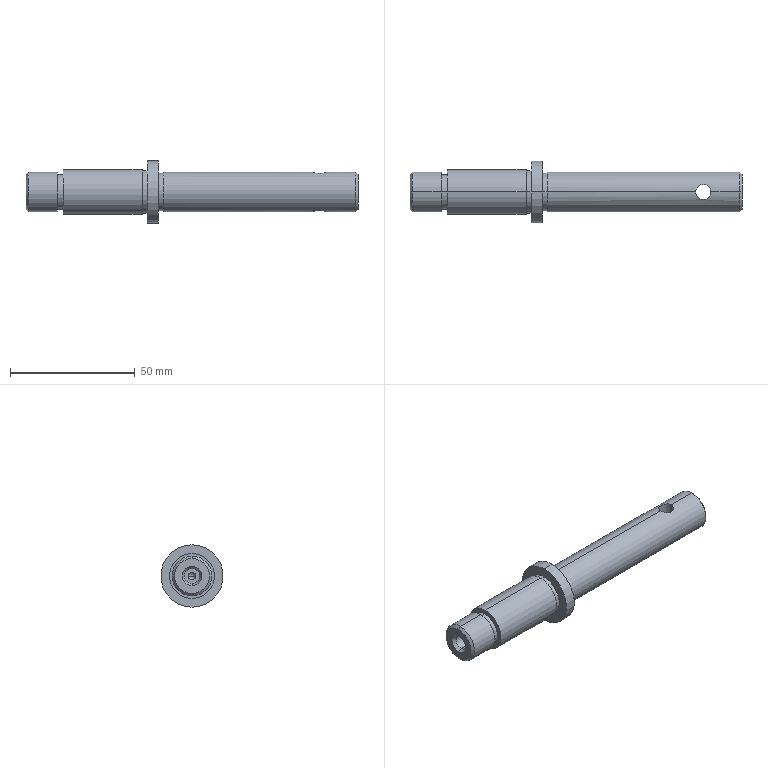Part | SolidWorks | features ICE 3, Chamfer 2, RevCut 1, Revolution 1 | 1 solid | 37 faces | box 133 x 25 x 25 mm | volume 28520 mm3 | cylinder 20 | plane 9 | cone 6 | sphere 2 | commonest cylinder face diameters 6 x4 16 x4 3 x2 14 x2 15 x2 17 x2
STEP:
#1=CARTESIAN_POINT('',(58.,-1.5,0.));
#2=VERTEX_POINT('',#1);
#3=CARTESIAN_POINT('',(58.,0.,-1.5));
#4=VERTEX_POINT('',#3);
#5=CARTESIAN_POINT('',(58.,0.,0.));
#6=DIRECTION('',(1.,0.,0.));
#7=DIRECTION('',(0.,0.,1.));
#8=AXIS2_PLACEMENT_3D('',#5,#6,#7);
#9=CIRCLE('',#8,1.5);
#10=EDGE_CURVE('',#2,#4,#9,.T.);
#11=ORIENTED_EDGE('',*,*,#10,.F.);
#12=CARTESIAN_POINT('',(58.,1.5,0.));
#13=VERTEX_POINT('',#12);
#14=CARTESIAN_POINT('',(58.,0.,0.));
#15=DIRECTION('',(0.,0.,1.));
#16=DIRECTION('',(1.,0.,0.));
#17=AXIS2_PLACEMENT_3D('',#14,#15,#16);
#18=CIRCLE('',#17,1.5);
#19=EDGE_CURVE('',#2,#13,#18,.T.);
#20=ORIENTED_EDGE('',*,*,#19,.T.);
#21=CARTESIAN_POINT('',(58.,0.,0.));
#22=DIRECTION('',(1.,0.,0.));
#23=DIRECTION('',(0.,0.,1.));
#24=AXIS2_PLACEMENT_3D('',#21,#22,#23);
#25=CIRCLE('',#24,1.5);
#26=EDGE_CURVE('',#4,#13,#25,.T.);
#27=ORIENTED_EDGE('',*,*,#26,.F.);
#28=EDGE_LOOP('',(#11,#20,#27));
#29=FACE_OUTER_BOUND('',#28,.T.);
#30=CARTESIAN_POINT('',(58.,0.,0.));
#31=DIRECTION('',(0.,0.,-1.));
#32=DIRECTION('',(1.,0.,0.));
#33=AXIS2_PLACEMENT_3D('',#30,#31,#32);
#34=SPHERICAL_SURFACE('',#33,1.5);
#35=ADVANCED_FACE('',(#29),#34,.F.);
#36=CARTESIAN_POINT('',(0.,0.,7.));
#37=VERTEX_POINT('',#36);
#38=CARTESIAN_POINT('',(0.,0.,-7.));
#39=VERTEX_POINT('',#38);
#40=CARTESIAN_POINT('',(0.,0.,0.));
#41=DIRECTION('',(-1.,0.,0.));
#42=DIRECTION('',(0.,0.,1.));
#43=AXIS2_PLACEMENT_3D('',#40,#41,#42);
#44=CIRCLE('',#43,7.);
#45=EDGE_CURVE('',#37,#39,#44,.T.);
#46=ORIENTED_EDGE('',*,*,#45,.F.);
#47=CARTESIAN_POINT('',(1.,0.,8.));
#48=VERTEX_POINT('',#47);
#49=CARTESIAN_POINT('',(1.,0.,8.));
#50=DIRECTION('',(0.7071,0.,0.7071));
#51=VECTOR('',#50,1000.);
#52=LINE('',#49,#51);
#53=EDGE_CURVE('',#37,#48,#52,.T.);
#54=ORIENTED_EDGE('',*,*,#53,.T.);
#55=CARTESIAN_POINT('',(1.,0.,-8.));
#56=VERTEX_POINT('',#55);
#57=CARTESIAN_POINT('',(1.,0.,0.));
#58=DIRECTION('',(1.,0.,0.));
#59=DIRECTION('',(0.,0.,1.));
#60=AXIS2_PLACEMENT_3D('',#57,#58,#59);
#61=CIRCLE('',#60,8.);
#62=EDGE_CURVE('',#56,#48,#61,.T.);
#63=ORIENTED_EDGE('',*,*,#62,.F.);
#64=CARTESIAN_POINT('',(1.,0.,-8.));
#65=DIRECTION('',(0.7071,0.,-0.7071));
#66=VECTOR('',#65,1000.);
#67=LINE('',#64,#66);
#68=EDGE_CURVE('',#39,#56,#67,.T.);
#69=ORIENTED_EDGE('',*,*,#68,.F.);
#70=EDGE_LOOP('',(#46,#54,#63,#69));
#71=FACE_OUTER_BOUND('',#70,.T.);
#72=CARTESIAN_POINT('',(1.,0.,0.));
#73=DIRECTION('',(1.,0.,0.));
#74=DIRECTION('',(0.,0.,-1.));
#75=AXIS2_PLACEMENT_3D('',#72,#73,#74);
#76=CONICAL_SURFACE('',#75,8.,0.7854);
#77=ADVANCED_FACE('',(#71),#76,.T.);
#78=CARTESIAN_POINT('',(133.,0.,-7.));
#79=VERTEX_POINT('',#78);
#80=CARTESIAN_POINT('',(133.,0.,7.));
#81=VERTEX_POINT('',#80);
#82=CARTESIAN_POINT('',(133.,0.,0.));
#83=DIRECTION('',(1.,0.,0.));
#84=DIRECTION('',(0.,0.,-1.));
#85=AXIS2_PLACEMENT_3D('',#82,#83,#84);
#86=CIRCLE('',#85,7.);
#87=EDGE_CURVE('',#79,#81,#86,.T.);
#88=ORIENTED_EDGE('',*,*,#87,.F.);
#89=CARTESIAN_POINT('',(132.,0.,-8.));
#90=VERTEX_POINT('',#89);
#91=CARTESIAN_POINT('',(133.,0.,-7.));
#92=DIRECTION('',(-0.7071,0.,-0.7071));
#93=VECTOR('',#92,1000.);
#94=LINE('',#91,#93);
#95=EDGE_CURVE('',#79,#90,#94,.T.);
#96=ORIENTED_EDGE('',*,*,#95,.T.);
#97=CARTESIAN_POINT('',(132.,0.,8.));
#98=VERTEX_POINT('',#97);
#99=CARTESIAN_POINT('',(132.,0.,0.));
#100=DIRECTION('',(-1.,0.,0.));
#101=DIRECTION('',(0.,0.,-1.));
#102=AXIS2_PLACEMENT_3D('',#99,#100,#101);
#103=CIRCLE('',#102,8.);
#104=EDGE_CURVE('',#98,#90,#103,.T.);
#105=ORIENTED_EDGE('',*,*,#104,.F.);
#106=CARTESIAN_POINT('',(133.,0.,7.));
#107=DIRECTION('',(-0.7071,0.,0.7071));
#108=VECTOR('',#107,1000.);
#109=LINE('',#106,#108);
#110=EDGE_CURVE('',#81,#98,#109,.T.);
#111=ORIENTED_EDGE('',*,*,#110,.F.);
#112=EDGE_LOOP('',(#88,#96,#105,#111));
#113=FACE_OUTER_BOUND('',#112,.T.);
#114=CARTESIAN_POINT('',(133.,0.,0.));
#115=DIRECTION('',(-1.,0.,0.));
#116=DIRECTION('',(0.,0.,1.));
#117=AXIS2_PLACEMENT_3D('',#114,#115,#116);
#118=CONICAL_SURFACE('',#117,7.,0.7854);
#119=ADVANCED_FACE('',(#113),#118,.T.);
#120=CARTESIAN_POINT('',(1.5,0.,-3.));
#121=VERTEX_POINT('',#120);
#122=CARTESIAN_POINT('',(1.5,0.,3.));
#123=VERTEX_POINT('',#122);
#124=CARTESIAN_POINT('',(1.5,0.,0.));
#125=DIRECTION('',(-1.,0.,0.));
#126=DIRECTION('',(0.,0.,1.));
#127=AXIS2_PLACEMENT_3D('',#124,#125,#126);
#128=CIRCLE('',#127,3.);
#129=EDGE_CURVE('',#121,#123,#128,.T.);
#130=ORIENTED_EDGE('',*,*,#129,.F.);
#131=CARTESIAN_POINT('',(0.,0.,-3.866));
#132=VERTEX_POINT('',#131);
#133=CARTESIAN_POINT('',(0.,0.,-3.866));
#134=DIRECTION('',(-0.866,0.,-0.5));
#135=VECTOR('',#134,1000.);
#136=LINE('',#133,#135);
#137=EDGE_CURVE('',#121,#132,#136,.T.);
#138=ORIENTED_EDGE('',*,*,#137,.T.);
#139=CARTESIAN_POINT('',(0.,0.,3.866));
#140=VERTEX_POINT('',#139);
#141=CARTESIAN_POINT('',(0.,0.,0.));
#142=DIRECTION('',(1.,0.,0.));
#143=DIRECTION('',(0.,0.,1.));
#144=AXIS2_PLACEMENT_3D('',#141,#142,#143);
#145=CIRCLE('',#144,3.866);
#146=EDGE_CURVE('',#140,#132,#145,.T.);
#147=ORIENTED_EDGE('',*,*,#146,.F.);
#148=CARTESIAN_POINT('',(0.,0.,3.866));
#149=DIRECTION('',(-0.866,0.,0.5));
#150=VECTOR('',#149,1000.);
#151=LINE('',#148,#150);
#152=EDGE_CURVE('',#123,#140,#151,.T.);
#153=ORIENTED_EDGE('',*,*,#152,.F.);
#154=EDGE_LOOP('',(#130,#138,#147,#153));
#155=FACE_OUTER_BOUND('',#154,.T.);
#156=CARTESIAN_POINT('',(0.,0.,0.));
#157=DIRECTION('',(-1.,0.,0.));
#158=DIRECTION('',(0.,0.,1.));
#159=AXIS2_PLACEMENT_3D('',#156,#157,#158);
#160=CONICAL_SURFACE('',#159,3.866,0.5236);
#161=ADVANCED_FACE('',(#155),#160,.F.);
#162=CARTESIAN_POINT('',(58.,0.,1.5));
#163=VERTEX_POINT('',#162);
#164=CARTESIAN_POINT('',(58.,0.,0.));
#165=DIRECTION('',(1.,0.,0.));
#166=DIRECTION('',(0.,0.,1.));
#167=AXIS2_PLACEMENT_3D('',#164,#165,#166);
#168=CIRCLE('',#167,1.5);
#169=EDGE_CURVE('',#163,#2,#168,.T.);
#170=ORIENTED_EDGE('',*,*,#169,.T.);
#171=ORIENTED_EDGE('',*,*,#10,.T.);
#172=CARTESIAN_POINT('',(8.,0.,-1.5));
#173=VERTEX_POINT('',#172);
#174=CARTESIAN_POINT('',(58.,0.,-1.5));
#175=DIRECTION('',(-1.,0.,0.));
#176=VECTOR('',#175,1000.);
#177=LINE('',#174,#176);
#178=EDGE_CURVE('',#4,#173,#177,.T.);
#179=ORIENTED_EDGE('',*,*,#178,.T.);
#180=CARTESIAN_POINT('',(8.,0.,1.5));
#181=VERTEX_POINT('',#180);
#182=CARTESIAN_POINT('',(8.,0.,0.));
#183=DIRECTION('',(-1.,0.,0.));
#184=DIRECTION('',(0.,0.,1.));
#185=AXIS2_PLACEMENT_3D('',#182,#183,#184);
#186=CIRCLE('',#185,1.5);
#187=EDGE_CURVE('',#173,#181,#186,.T.);
#188=ORIENTED_EDGE('',*,*,#187,.T.);
#189=CARTESIAN_POINT('',(58.,0.,1.5));
#190=DIRECTION('',(-1.,0.,0.));
#191=VECTOR('',#190,1000.);
#192=LINE('',#189,#191);
#193=EDGE_CURVE('',#163,#181,#192,.T.);
#194=ORIENTED_EDGE('',*,*,#193,.F.);
#195=EDGE_LOOP('',(#170,#171,#179,#188,#194));
#196=FACE_OUTER_BOUND('',#195,.T.);
#197=CARTESIAN_POINT('',(58.,0.,0.));
#198=DIRECTION('',(-1.,0.,0.));
#199=DIRECTION('',(0.,0.,1.));
#200=AXIS2_PLACEMENT_3D('',#197,#198,#199);
#201=CYLINDRICAL_SURFACE('',#200,1.5);
#202=ADVANCED_FACE('',(#196),#201,.F.);
#203=ORIENTED_EDGE('',*,*,#129,.T.);
#204=CARTESIAN_POINT('',(8.,0.,3.));
#205=VERTEX_POINT('',#204);
#206=CARTESIAN_POINT('',(-0.000012,0.,3.));
#207=DIRECTION('',(1.,0.,0.));
#208=VECTOR('',#207,1000.);
#209=LINE('',#206,#208);
#210=EDGE_CURVE('',#123,#205,#209,.T.);
#211=ORIENTED_EDGE('',*,*,#210,.T.);
#212=CARTESIAN_POINT('',(8.,0.,-3.));
#213=VERTEX_POINT('',#212);
#214=CARTESIAN_POINT('',(8.,0.,0.));
#215=DIRECTION('',(-1.,0.,0.));
#216=DIRECTION('',(0.,0.,1.));
#217=AXIS2_PLACEMENT_3D('',#214,#215,#216);
#218=CIRCLE('',#217,3.);
#219=EDGE_CURVE('',#213,#205,#218,.T.);
#220=ORIENTED_EDGE('',*,*,#219,.F.);
#221=CARTESIAN_POINT('',(-0.000012,0.,-3.));
#222=DIRECTION('',(1.,0.,0.));
#223=VECTOR('',#222,1000.);
#224=LINE('',#221,#223);
#225=EDGE_CURVE('',#121,#213,#224,.T.);
#226=ORIENTED_EDGE('',*,*,#225,.F.);
#227=EDGE_LOOP('',(#203,#211,#220,#226));
#228=FACE_OUTER_BOUND('',#227,.T.);
#229=CARTESIAN_POINT('',(-0.000012,0.,0.));
#230=DIRECTION('',(1.,0.,0.));
#231=DIRECTION('',(0.,0.,-1.));
#232=AXIS2_PLACEMENT_3D('',#229,#230,#231);
#233=CYLINDRICAL_SURFACE('',#232,3.);
#234=ADVANCED_FACE('',(#228),#233,.F.);
#235=CARTESIAN_POINT('',(120.5,0.,-8.));
#236=VERTEX_POINT('',#235);
#237=CARTESIAN_POINT('',(114.5,0.,-8.));
#238=VERTEX_POINT('',#237);
#239=CARTESIAN_POINT('',(120.5,0.,-8.));
#240=CARTESIAN_POINT('',(120.5,-0.1971,-8.));
#241=CARTESIAN_POINT('',(120.48,-0.3965,-7.993));
#242=CARTESIAN_POINT('',(120.402,-0.7855,-7.964));
#243=CARTESIAN_POINT('',(120.345,-0.9732,-7.943));
#244=CARTESIAN_POINT('',(120.193,-1.336,-7.89));
#245=CARTESIAN_POINT('',(120.099,-1.511,-7.858));
#246=CARTESIAN_POINT('',(119.882,-1.834,-7.789));
#247=CARTESIAN_POINT('',(119.759,-1.984,-7.751));
#248=CARTESIAN_POINT('',(119.481,-2.261,-7.675));
#249=CARTESIAN_POINT('',(119.331,-2.385,-7.637));
#250=CARTESIAN_POINT('',(119.008,-2.601,-7.566));
#251=CARTESIAN_POINT('',(118.834,-2.694,-7.533));
#252=CARTESIAN_POINT('',(118.471,-2.845,-7.477));
#253=CARTESIAN_POINT('',(118.283,-2.903,-7.455));
#254=CARTESIAN_POINT('',(117.897,-2.98,-7.424));
#255=CARTESIAN_POINT('',(117.696,-3.,-7.416));
#256=CARTESIAN_POINT('',(117.301,-3.,-7.416));
#257=CARTESIAN_POINT('',(117.105,-2.98,-7.424));
#258=CARTESIAN_POINT('',(116.715,-2.902,-7.455));
#259=CARTESIAN_POINT('',(116.525,-2.844,-7.478));
#260=CARTESIAN_POINT('',(116.164,-2.693,-7.533));
#261=CARTESIAN_POINT('',(115.99,-2.6,-7.567));
#262=CARTESIAN_POINT('',(115.665,-2.382,-7.638));
#263=CARTESIAN_POINT('',(115.516,-2.258,-7.676));
#264=CARTESIAN_POINT('',(115.241,-1.983,-7.752));
#265=CARTESIAN_POINT('',(115.115,-1.83,-7.79));
#266=CARTESIAN_POINT('',(114.899,-1.507,-7.859));
#267=CARTESIAN_POINT('',(114.806,-1.336,-7.89));
#268=CARTESIAN_POINT('',(114.655,-0.9711,-7.943));
#269=CARTESIAN_POINT('',(114.597,-0.781,-7.964));
#270=CARTESIAN_POINT('',(114.52,-0.3964,-7.992));
#271=CARTESIAN_POINT('',(114.5,-0.2002,-8.));
#272=CARTESIAN_POINT('',(114.5,0.,-8.));
#273=B_SPLINE_CURVE_WITH_KNOTS('',3,(#239,#240,#241,#242,#243,#244,#245,#246,#247,#248,#249,#250,#251,#252,#253,#254,#255,#256,#257,#258,#259,#260,#261,#262,#263,#264,#265,#266,#267,#268,#269,#270,#271,#272),.UNSPECIFIED.,.F.,.F.,(4,2,2,2,2,2,2,2,2,2,2,2,2,2,2,2,4),(0.009467,0.01006,0.01065,0.01124,0.01183,0.01242,0.01302,0.01361,0.0142,0.01479,0.01538,0.01597,0.01657,0.01716,0.01775,0.01834,0.01893),.UNSPECIFIED.);
#274=EDGE_CURVE('',#236,#238,#273,.T.);
#275=ORIENTED_EDGE('',*,*,#274,.T.);
#276=CARTESIAN_POINT('',(114.5,0.,8.));
#277=VERTEX_POINT('',#276);
#278=CARTESIAN_POINT('',(114.5,0.,-12.5));
#279=DIRECTION('',(0.,0.,1.));
#280=VECTOR('',#279,1000.);
#281=LINE('',#278,#280);
#282=EDGE_CURVE('',#238,#277,#281,.T.);
#283=ORIENTED_EDGE('',*,*,#282,.T.);
#284=CARTESIAN_POINT('',(120.5,0.,8.));
#285=VERTEX_POINT('',#284);
#286=CARTESIAN_POINT('',(114.5,0.,8.));
#287=CARTESIAN_POINT('',(114.5,-0.1971,8.));
#288=CARTESIAN_POINT('',(114.52,-0.3965,7.993));
#289=CARTESIAN_POINT('',(114.598,-0.7855,7.964));
#290=CARTESIAN_POINT('',(114.655,-0.9732,7.943));
#291=CARTESIAN_POINT('',(114.807,-1.336,7.89));
#292=CARTESIAN_POINT('',(114.901,-1.511,7.858));
#293=CARTESIAN_POINT('',(115.118,-1.834,7.789));
#294=CARTESIAN_POINT('',(115.241,-1.984,7.751));
#295=CARTESIAN_POINT('',(115.519,-2.261,7.675));
#296=CARTESIAN_POINT('',(115.669,-2.385,7.637));
#297=CARTESIAN_POINT('',(115.992,-2.601,7.566));
#298=CARTESIAN_POINT('',(116.166,-2.694,7.533));
#299=CARTESIAN_POINT('',(116.529,-2.845,7.477));
#300=CARTESIAN_POINT('',(116.717,-2.903,7.455));
#301=CARTESIAN_POINT('',(117.103,-2.98,7.424));
#302=CARTESIAN_POINT('',(117.304,-3.,7.416));
#303=CARTESIAN_POINT('',(117.699,-3.,7.416));
#304=CARTESIAN_POINT('',(117.895,-2.98,7.424));
#305=CARTESIAN_POINT('',(118.285,-2.902,7.455));
#306=CARTESIAN_POINT('',(118.475,-2.844,7.478));
#307=CARTESIAN_POINT('',(118.836,-2.693,7.533));
#308=CARTESIAN_POINT('',(119.01,-2.6,7.567));
#309=CARTESIAN_POINT('',(119.335,-2.382,7.638));
#310=CARTESIAN_POINT('',(119.484,-2.258,7.676));
#311=CARTESIAN_POINT('',(119.759,-1.983,7.752));
#312=CARTESIAN_POINT('',(119.885,-1.83,7.79));
#313=CARTESIAN_POINT('',(120.101,-1.507,7.859));
#314=CARTESIAN_POINT('',(120.194,-1.336,7.89));
#315=CARTESIAN_POINT('',(120.345,-0.9711,7.943));
#316=CARTESIAN_POINT('',(120.403,-0.781,7.964));
#317=CARTESIAN_POINT('',(120.48,-0.3964,7.992));
#318=CARTESIAN_POINT('',(120.5,-0.2002,8.));
#319=CARTESIAN_POINT('',(120.5,0.,8.));
#320=B_SPLINE_CURVE_WITH_KNOTS('',3,(#286,#287,#288,#289,#290,#291,#292,#293,#294,#295,#296,#297,#298,#299,#300,#301,#302,#303,#304,#305,#306,#307,#308,#309,#310,#311,#312,#313,#314,#315,#316,#317,#318,#319),.UNSPECIFIED.,.F.,.F.,(4,2,2,2,2,2,2,2,2,2,2,2,2,2,2,2,4),(0.009467,0.01006,0.01065,0.01124,0.01183,0.01242,0.01302,0.01361,0.0142,0.01479,0.01538,0.01597,0.01657,0.01716,0.01775,0.01834,0.01893),.UNSPECIFIED.);
#321=EDGE_CURVE('',#277,#285,#320,.T.);
#322=ORIENTED_EDGE('',*,*,#321,.T.);
#323=CARTESIAN_POINT('',(120.5,0.,-12.5));
#324=DIRECTION('',(0.,0.,1.));
#325=VECTOR('',#324,1000.);
#326=LINE('',#323,#325);
#327=EDGE_CURVE('',#236,#285,#326,.T.);
#328=ORIENTED_EDGE('',*,*,#327,.F.);
#329=EDGE_LOOP('',(#275,#283,#322,#328));
#330=FACE_OUTER_BOUND('',#329,.T.);
#331=CARTESIAN_POINT('',(117.5,0.,-12.5));
#332=DIRECTION('',(0.,0.,1.));
#333=DIRECTION('',(1.,0.,0.));
#334=AXIS2_PLACEMENT_3D('',#331,#332,#333);
#335=CYLINDRICAL_SURFACE('',#334,3.);
#336=ADVANCED_FACE('',(#330),#335,.F.);
#337=CARTESIAN_POINT('',(55.,0.,-8.));
#338=VERTEX_POINT('',#337);
#339=CARTESIAN_POINT('',(55.,0.,8.));
#340=VERTEX_POINT('',#339);
#341=CARTESIAN_POINT('',(55.,0.,0.));
#342=DIRECTION('',(1.,0.,0.));
#343=DIRECTION('',(0.,0.,-1.));
#344=AXIS2_PLACEMENT_3D('',#341,#342,#343);
#345=CIRCLE('',#344,8.);
#346=EDGE_CURVE('',#338,#340,#345,.T.);
#347=ORIENTED_EDGE('',*,*,#346,.T.);
#348=CARTESIAN_POINT('',(133.,0.,8.));
#349=DIRECTION('',(1.,0.,0.));
#350=VECTOR('',#349,1000.);
#351=LINE('',#348,#350);
#352=EDGE_CURVE('',#340,#277,#351,.T.);
#353=ORIENTED_EDGE('',*,*,#352,.T.);
#354=CARTESIAN_POINT('',(120.5,0.,8.));
#355=CARTESIAN_POINT('',(120.5,0.2002,8.));
#356=CARTESIAN_POINT('',(120.48,0.3967,7.993));
#357=CARTESIAN_POINT('',(120.403,0.7827,7.964));
#358=CARTESIAN_POINT('',(120.344,0.9743,7.943));
#359=CARTESIAN_POINT('',(120.193,1.337,7.89));
#360=CARTESIAN_POINT('',(120.1,1.509,7.858));
#361=CARTESIAN_POINT('',(119.883,1.833,7.789));
#362=CARTESIAN_POINT('',(119.757,1.986,7.751));
#363=CARTESIAN_POINT('',(119.346,2.396,7.638));
#364=CARTESIAN_POINT('',(119.015,2.619,7.561));
#365=CARTESIAN_POINT('',(118.474,2.844,7.478));
#366=CARTESIAN_POINT('',(118.283,2.903,7.455));
#367=CARTESIAN_POINT('',(117.895,2.98,7.424));
#368=CARTESIAN_POINT('',(117.699,3.,7.416));
#369=CARTESIAN_POINT('',(117.304,3.,7.416));
#370=CARTESIAN_POINT('',(117.103,2.98,7.424));
#371=CARTESIAN_POINT('',(116.717,2.903,7.455));
#372=CARTESIAN_POINT('',(116.529,2.845,7.477));
#373=CARTESIAN_POINT('',(116.163,2.693,7.534));
#374=CARTESIAN_POINT('',(115.991,2.6,7.566));
#375=CARTESIAN_POINT('',(115.668,2.384,7.637));
#376=CARTESIAN_POINT('',(115.515,2.258,7.676));
#377=CARTESIAN_POINT('',(115.24,1.983,7.752));
#378=CARTESIAN_POINT('',(115.117,1.833,7.789));
#379=CARTESIAN_POINT('',(114.9,1.509,7.858));
#380=CARTESIAN_POINT('',(114.806,1.334,7.89));
#381=CARTESIAN_POINT('',(114.655,0.973,7.943));
#382=CARTESIAN_POINT('',(114.598,0.7855,7.964));
#383=CARTESIAN_POINT('',(114.52,0.3956,7.993));
#384=CARTESIAN_POINT('',(114.5,0.1972,8.));
#385=CARTESIAN_POINT('',(114.5,0.,8.));
#386=B_SPLINE_CURVE_WITH_KNOTS('',3,(#354,#355,#356,#357,#358,#359,#360,#361,#362,#363,#364,#365,#366,#367,#368,#369,#370,#371,#372,#373,#374,#375,#376,#377,#378,#379,#380,#381,#382,#383,#384,#385),.UNSPECIFIED.,.F.,.F.,(4,2,2,2,2,2,2,2,2,2,2,2,2,2,2,4),(0.,0.0005917,0.001183,0.001775,0.002367,0.00355,0.004142,0.004733,0.005325,0.005917,0.006508,0.0071,0.007692,0.008283,0.008875,0.009467),.UNSPECIFIED.);
#387=EDGE_CURVE('',#285,#277,#386,.T.);
#388=ORIENTED_EDGE('',*,*,#387,.F.);
#389=CARTESIAN_POINT('',(133.,0.,8.));
#390=DIRECTION('',(1.,0.,0.));
#391=VECTOR('',#390,1000.);
#392=LINE('',#389,#391);
#393=EDGE_CURVE('',#285,#98,#392,.T.);
#394=ORIENTED_EDGE('',*,*,#393,.T.);
#395=ORIENTED_EDGE('',*,*,#104,.T.);
#396=CARTESIAN_POINT('',(133.,0.,-8.));
#397=DIRECTION('',(1.,0.,0.));
#398=VECTOR('',#397,1000.);
#399=LINE('',#396,#398);
#400=EDGE_CURVE('',#236,#90,#399,.T.);
#401=ORIENTED_EDGE('',*,*,#400,.F.);
#402=CARTESIAN_POINT('',(114.5,0.,-8.));
#403=CARTESIAN_POINT('',(114.5,0.2002,-8.));
#404=CARTESIAN_POINT('',(114.52,0.3967,-7.993));
#405=CARTESIAN_POINT('',(114.597,0.7827,-7.964));
#406=CARTESIAN_POINT('',(114.656,0.9743,-7.943));
#407=CARTESIAN_POINT('',(114.807,1.337,-7.89));
#408=CARTESIAN_POINT('',(114.9,1.509,-7.858));
#409=CARTESIAN_POINT('',(115.117,1.833,-7.789));
#410=CARTESIAN_POINT('',(115.243,1.986,-7.751));
#411=CARTESIAN_POINT('',(115.654,2.396,-7.638));
#412=CARTESIAN_POINT('',(115.985,2.619,-7.561));
#413=CARTESIAN_POINT('',(116.526,2.844,-7.478));
#414=CARTESIAN_POINT('',(116.717,2.903,-7.455));
#415=CARTESIAN_POINT('',(117.105,2.98,-7.424));
#416=CARTESIAN_POINT('',(117.301,3.,-7.416));
#417=CARTESIAN_POINT('',(117.696,3.,-7.416));
#418=CARTESIAN_POINT('',(117.897,2.98,-7.424));
#419=CARTESIAN_POINT('',(118.283,2.903,-7.455));
#420=CARTESIAN_POINT('',(118.471,2.845,-7.477));
#421=CARTESIAN_POINT('',(118.837,2.693,-7.534));
#422=CARTESIAN_POINT('',(119.009,2.6,-7.566));
#423=CARTESIAN_POINT('',(119.332,2.384,-7.637));
#424=CARTESIAN_POINT('',(119.485,2.258,-7.676));
#425=CARTESIAN_POINT('',(119.76,1.983,-7.752));
#426=CARTESIAN_POINT('',(119.883,1.833,-7.789));
#427=CARTESIAN_POINT('',(120.1,1.509,-7.858));
#428=CARTESIAN_POINT('',(120.194,1.334,-7.89));
#429=CARTESIAN_POINT('',(120.345,0.973,-7.943));
#430=CARTESIAN_POINT('',(120.402,0.7855,-7.964));
#431=CARTESIAN_POINT('',(120.48,0.3956,-7.993));
#432=CARTESIAN_POINT('',(120.5,0.1972,-8.));
#433=CARTESIAN_POINT('',(120.5,0.,-8.));
#434=B_SPLINE_CURVE_WITH_KNOTS('',3,(#402,#403,#404,#405,#406,#407,#408,#409,#410,#411,#412,#413,#414,#415,#416,#417,#418,#419,#420,#421,#422,#423,#424,#425,#426,#427,#428,#429,#430,#431,#432,#433),.UNSPECIFIED.,.F.,.F.,(4,2,2,2,2,2,2,2,2,2,2,2,2,2,2,4),(0.,0.0005917,0.001183,0.001775,0.002367,0.00355,0.004142,0.004733,0.005325,0.005917,0.006508,0.0071,0.007692,0.008283,0.008875,0.009467),.UNSPECIFIED.);
#435=EDGE_CURVE('',#238,#236,#434,.T.);
#436=ORIENTED_EDGE('',*,*,#435,.F.);
#437=CARTESIAN_POINT('',(133.,0.,-8.));
#438=DIRECTION('',(1.,0.,0.));
#439=VECTOR('',#438,1000.);
#440=LINE('',#437,#439);
#441=EDGE_CURVE('',#338,#238,#440,.T.);
#442=ORIENTED_EDGE('',*,*,#441,.F.);
#443=EDGE_LOOP('',(#347,#353,#388,#394,#395,#401,#436,#442));
#444=FACE_OUTER_BOUND('',#443,.T.);
#445=CARTESIAN_POINT('',(133.,0.,0.));
#446=DIRECTION('',(1.,0.,0.));
#447=DIRECTION('',(0.,0.,-1.));
#448=AXIS2_PLACEMENT_3D('',#445,#446,#447);
#449=CYLINDRICAL_SURFACE('',#448,8.);
#450=ADVANCED_FACE('',(#444),#449,.T.);
#451=CARTESIAN_POINT('',(53.,0.,-7.5));
#452=VERTEX_POINT('',#451);
#453=CARTESIAN_POINT('',(53.,0.,7.5));
#454=VERTEX_POINT('',#453);
#455=CARTESIAN_POINT('',(53.,0.,0.));
#456=DIRECTION('',(1.,0.,0.));
#457=DIRECTION('',(0.,0.,-1.));
#458=AXIS2_PLACEMENT_3D('',#455,#456,#457);
#459=CIRCLE('',#458,7.5);
#460=EDGE_CURVE('',#452,#454,#459,.T.);
#461=ORIENTED_EDGE('',*,*,#460,.T.);
#462=CARTESIAN_POINT('',(55.,0.,7.5));
#463=VERTEX_POINT('',#462);
#464=CARTESIAN_POINT('',(133.,0.,7.5));
#465=DIRECTION('',(1.,0.,0.));
#466=VECTOR('',#465,1000.);
#467=LINE('',#464,#466);
#468=EDGE_CURVE('',#454,#463,#467,.T.);
#469=ORIENTED_EDGE('',*,*,#468,.T.);
#470=CARTESIAN_POINT('',(55.,0.,-7.5));
#471=VERTEX_POINT('',#470);
#472=CARTESIAN_POINT('',(55.,0.,0.));
#473=DIRECTION('',(1.,0.,0.));
#474=DIRECTION('',(0.,0.,-1.));
#475=AXIS2_PLACEMENT_3D('',#472,#473,#474);
#476=CIRCLE('',#475,7.5);
#477=EDGE_CURVE('',#471,#463,#476,.T.);
#478=ORIENTED_EDGE('',*,*,#477,.F.);
#479=CARTESIAN_POINT('',(133.,0.,-7.5));
#480=DIRECTION('',(1.,0.,0.));
#481=VECTOR('',#480,1000.);
#482=LINE('',#479,#481);
#483=EDGE_CURVE('',#452,#471,#482,.T.);
#484=ORIENTED_EDGE('',*,*,#483,.F.);
#485=EDGE_LOOP('',(#461,#469,#478,#484));
#486=FACE_OUTER_BOUND('',#485,.T.);
#487=CARTESIAN_POINT('',(133.,0.,0.));
#488=DIRECTION('',(1.,0.,0.));
#489=DIRECTION('',(0.,0.,-1.));
#490=AXIS2_PLACEMENT_3D('',#487,#488,#489);
#491=CYLINDRICAL_SURFACE('',#490,7.5);
#492=ADVANCED_FACE('',(#486),#491,.T.);
#493=CARTESIAN_POINT('',(48.5,0.,-12.5));
#494=VERTEX_POINT('',#493);
#495=CARTESIAN_POINT('',(48.5,0.,12.5));
#496=VERTEX_POINT('',#495);
#497=CARTESIAN_POINT('',(48.5,0.,0.));
#498=DIRECTION('',(1.,0.,0.));
#499=DIRECTION('',(0.,0.,-1.));
#500=AXIS2_PLACEMENT_3D('',#497,#498,#499);
#501=CIRCLE('',#500,12.5);
#502=EDGE_CURVE('',#494,#496,#501,.T.);
#503=ORIENTED_EDGE('',*,*,#502,.T.);
#504=CARTESIAN_POINT('',(53.,0.,12.5));
#505=VERTEX_POINT('',#504);
#506=CARTESIAN_POINT('',(133.,0.,12.5));
#507=DIRECTION('',(1.,0.,0.));
#508=VECTOR('',#507,1000.);
#509=LINE('',#506,#508);
#510=EDGE_CURVE('',#496,#505,#509,.T.);
#511=ORIENTED_EDGE('',*,*,#510,.T.);
#512=CARTESIAN_POINT('',(53.,0.,-12.5));
#513=VERTEX_POINT('',#512);
#514=CARTESIAN_POINT('',(53.,0.,0.));
#515=DIRECTION('',(1.,0.,0.));
#516=DIRECTION('',(0.,0.,-1.));
#517=AXIS2_PLACEMENT_3D('',#514,#515,#516);
#518=CIRCLE('',#517,12.5);
#519=EDGE_CURVE('',#513,#505,#518,.T.);
#520=ORIENTED_EDGE('',*,*,#519,.F.);
#521=CARTESIAN_POINT('',(133.,0.,-12.5));
#522=DIRECTION('',(1.,0.,0.));
#523=VECTOR('',#522,1000.);
#524=LINE('',#521,#523);
#525=EDGE_CURVE('',#494,#513,#524,.T.);
#526=ORIENTED_EDGE('',*,*,#525,.F.);
#527=EDGE_LOOP('',(#503,#511,#520,#526));
#528=FACE_OUTER_BOUND('',#527,.T.);
#529=CARTESIAN_POINT('',(133.,0.,0.));
#530=DIRECTION('',(1.,0.,0.));
#531=DIRECTION('',(0.,0.,-1.));
#532=AXIS2_PLACEMENT_3D('',#529,#530,#531);
#533=CYLINDRICAL_SURFACE('',#532,12.5);
#534=ADVANCED_FACE('',(#528),#533,.T.);
#535=CARTESIAN_POINT('',(46.5,0.,-8.5));
#536=VERTEX_POINT('',#535);
#537=CARTESIAN_POINT('',(46.5,0.,8.5));
#538=VERTEX_POINT('',#537);
#539=CARTESIAN_POINT('',(46.5,0.,0.));
#540=DIRECTION('',(1.,0.,0.));
#541=DIRECTION('',(0.,0.,-1.));
#542=AXIS2_PLACEMENT_3D('',#539,#540,#541);
#543=CIRCLE('',#542,8.5);
#544=EDGE_CURVE('',#536,#538,#543,.T.);
#545=ORIENTED_EDGE('',*,*,#544,.T.);
#546=CARTESIAN_POINT('',(48.5,0.,8.5));
#547=VERTEX_POINT('',#546);
#548=CARTESIAN_POINT('',(133.,0.,8.5));
#549=DIRECTION('',(1.,0.,0.));
#550=VECTOR('',#549,1000.);
#551=LINE('',#548,#550);
#552=EDGE_CURVE('',#538,#547,#551,.T.);
#553=ORIENTED_EDGE('',*,*,#552,.T.);
#554=CARTESIAN_POINT('',(48.5,0.,-8.5));
#555=VERTEX_POINT('',#554);
#556=CARTESIAN_POINT('',(48.5,0.,0.));
#557=DIRECTION('',(1.,0.,0.));
#558=DIRECTION('',(0.,0.,-1.));
#559=AXIS2_PLACEMENT_3D('',#556,#557,#558);
#560=CIRCLE('',#559,8.5);
#561=EDGE_CURVE('',#555,#547,#560,.T.);
#562=ORIENTED_EDGE('',*,*,#561,.F.);
#563=CARTESIAN_POINT('',(133.,0.,-8.5));
#564=DIRECTION('',(1.,0.,0.));
#565=VECTOR('',#564,1000.);
#566=LINE('',#563,#565);
#567=EDGE_CURVE('',#536,#555,#566,.T.);
#568=ORIENTED_EDGE('',*,*,#567,.F.);
#569=EDGE_LOOP('',(#545,#553,#562,#568));
#570=FACE_OUTER_BOUND('',#569,.T.);
#571=CARTESIAN_POINT('',(133.,0.,0.));
#572=DIRECTION('',(1.,0.,0.));
#573=DIRECTION('',(0.,0.,-1.));
#574=AXIS2_PLACEMENT_3D('',#571,#572,#573);
#575=CYLINDRICAL_SURFACE('',#574,8.5);
#576=ADVANCED_FACE('',(#570),#575,.T.);
#577=CARTESIAN_POINT('',(15.,0.,-9.));
#578=VERTEX_POINT('',#577);
#579=CARTESIAN_POINT('',(15.,0.,9.));
#580=VERTEX_POINT('',#579);
#581=CARTESIAN_POINT('',(15.,0.,0.));
#582=DIRECTION('',(1.,0.,0.));
#583=DIRECTION('',(0.,0.,-1.));
#584=AXIS2_PLACEMENT_3D('',#581,#582,#583);
#585=CIRCLE('',#584,9.);
#586=EDGE_CURVE('',#578,#580,#585,.T.);
#587=ORIENTED_EDGE('',*,*,#586,.T.);
#588=CARTESIAN_POINT('',(46.5,0.,9.));
#589=VERTEX_POINT('',#588);
#590=CARTESIAN_POINT('',(133.,0.,9.));
#591=DIRECTION('',(1.,0.,0.));
#592=VECTOR('',#591,1000.);
#593=LINE('',#590,#592);
#594=EDGE_CURVE('',#580,#589,#593,.T.);
#595=ORIENTED_EDGE('',*,*,#594,.T.);
#596=CARTESIAN_POINT('',(46.5,0.,-9.));
#597=VERTEX_POINT('',#596);
#598=CARTESIAN_POINT('',(46.5,0.,0.));
#599=DIRECTION('',(1.,0.,0.));
#600=DIRECTION('',(0.,0.,-1.));
#601=AXIS2_PLACEMENT_3D('',#598,#599,#600);
#602=CIRCLE('',#601,9.);
#603=EDGE_CURVE('',#597,#589,#602,.T.);
#604=ORIENTED_EDGE('',*,*,#603,.F.);
#605=CARTESIAN_POINT('',(133.,0.,-9.));
#606=DIRECTION('',(1.,0.,0.));
#607=VECTOR('',#606,1000.);
#608=LINE('',#605,#607);
#609=EDGE_CURVE('',#578,#597,#608,.T.);
#610=ORIENTED_EDGE('',*,*,#609,.F.);
#611=EDGE_LOOP('',(#587,#595,#604,#610));
#612=FACE_OUTER_BOUND('',#611,.T.);
#613=CARTESIAN_POINT('',(133.,0.,0.));
#614=DIRECTION('',(1.,0.,0.));
#615=DIRECTION('',(0.,0.,-1.));
#616=AXIS2_PLACEMENT_3D('',#613,#614,#615);
#617=CYLINDRICAL_SURFACE('',#616,9.);
#618=ADVANCED_FACE('',(#612),#617,.T.);
#619=CARTESIAN_POINT('',(12.5,0.,-7.));
#620=VERTEX_POINT('',#619);
#621=CARTESIAN_POINT('',(12.5,0.,7.));
#622=VERTEX_POINT('',#621);
#623=CARTESIAN_POINT('',(12.5,0.,0.));
#624=DIRECTION('',(1.,0.,0.));
#625=DIRECTION('',(0.,0.,-1.));
#626=AXIS2_PLACEMENT_3D('',#623,#624,#625);
#627=CIRCLE('',#626,7.);
#628=EDGE_CURVE('',#620,#622,#627,.T.);
#629=ORIENTED_EDGE('',*,*,#628,.T.);
#630=CARTESIAN_POINT('',(15.,0.,7.));
#631=VERTEX_POINT('',#630);
#632=CARTESIAN_POINT('',(133.,0.,7.));
#633=DIRECTION('',(1.,0.,0.));
#634=VECTOR('',#633,1000.);
#635=LINE('',#632,#634);
#636=EDGE_CURVE('',#622,#631,#635,.T.);
#637=ORIENTED_EDGE('',*,*,#636,.T.);
#638=CARTESIAN_POINT('',(15.,0.,-7.));
#639=VERTEX_POINT('',#638);
#640=CARTESIAN_POINT('',(15.,0.,0.));
#641=DIRECTION('',(1.,0.,0.));
#642=DIRECTION('',(0.,0.,-1.));
#643=AXIS2_PLACEMENT_3D('',#640,#641,#642);
#644=CIRCLE('',#643,7.);
#645=EDGE_CURVE('',#639,#631,#644,.T.);
#646=ORIENTED_EDGE('',*,*,#645,.F.);
#647=CARTESIAN_POINT('',(133.,0.,-7.));
#648=DIRECTION('',(1.,0.,0.));
#649=VECTOR('',#648,1000.);
#650=LINE('',#647,#649);
#651=EDGE_CURVE('',#620,#639,#650,.T.);
#652=ORIENTED_EDGE('',*,*,#651,.F.);
#653=EDGE_LOOP('',(#629,#637,#646,#652));
#654=FACE_OUTER_BOUND('',#653,.T.);
#655=CARTESIAN_POINT('',(133.,0.,0.));
#656=DIRECTION('',(1.,0.,0.));
#657=DIRECTION('',(0.,0.,-1.));
#658=AXIS2_PLACEMENT_3D('',#655,#656,#657);
#659=CYLINDRICAL_SURFACE('',#658,7.);
#660=ADVANCED_FACE('',(#654),#659,.T.);
#661=ORIENTED_EDGE('',*,*,#62,.T.);
#662=CARTESIAN_POINT('',(12.5,0.,8.));
#663=VERTEX_POINT('',#662);
#664=CARTESIAN_POINT('',(133.,0.,8.));
#665=DIRECTION('',(1.,0.,0.));
#666=VECTOR('',#665,1000.);
#667=LINE('',#664,#666);
#668=EDGE_CURVE('',#48,#663,#667,.T.);
#669=ORIENTED_EDGE('',*,*,#668,.T.);
#670=CARTESIAN_POINT('',(12.5,0.,-8.));
#671=VERTEX_POINT('',#670);
#672=CARTESIAN_POINT('',(12.5,0.,0.));
#673=DIRECTION('',(1.,0.,0.));
#674=DIRECTION('',(0.,0.,-1.));
#675=AXIS2_PLACEMENT_3D('',#672,#673,#674);
#676=CIRCLE('',#675,8.);
#677=EDGE_CURVE('',#671,#663,#676,.T.);
#678=ORIENTED_EDGE('',*,*,#677,.F.);
#679=CARTESIAN_POINT('',(133.,0.,-8.));
#680=DIRECTION('',(1.,0.,0.));
#681=VECTOR('',#680,1000.);
#682=LINE('',#679,#681);
#683=EDGE_CURVE('',#56,#671,#682,.T.);
#684=ORIENTED_EDGE('',*,*,#683,.F.);
#685=EDGE_LOOP('',(#661,#669,#678,#684));
#686=FACE_OUTER_BOUND('',#685,.T.);
#687=CARTESIAN_POINT('',(133.,0.,0.));
#688=DIRECTION('',(1.,0.,0.));
#689=DIRECTION('',(0.,0.,-1.));
#690=AXIS2_PLACEMENT_3D('',#687,#688,#689);
#691=CYLINDRICAL_SURFACE('',#690,8.);
#692=ADVANCED_FACE('',(#686),#691,.T.);
#693=CARTESIAN_POINT('',(0.,0.,0.));
#694=DIRECTION('',(-1.,0.,0.));
#695=DIRECTION('',(0.,0.,1.));
#696=AXIS2_PLACEMENT_3D('',#693,#694,#695);
#697=CIRCLE('',#696,7.);
#698=EDGE_CURVE('',#39,#37,#697,.T.);
#699=ORIENTED_EDGE('',*,*,#698,.T.);
#700=ORIENTED_EDGE('',*,*,#45,.T.);
#701=EDGE_LOOP('',(#699,#700));
#702=FACE_OUTER_BOUND('',#701,.T.);
#703=ORIENTED_EDGE('',*,*,#146,.T.);
#704=CARTESIAN_POINT('',(0.,0.,0.));
#705=DIRECTION('',(1.,0.,0.));
#706=DIRECTION('',(0.,0.,1.));
#707=AXIS2_PLACEMENT_3D('',#704,#705,#706);
#708=CIRCLE('',#707,3.866);
#709=EDGE_CURVE('',#132,#140,#708,.T.);
#710=ORIENTED_EDGE('',*,*,#709,.T.);
#711=EDGE_LOOP('',(#703,#710));
#712=FACE_BOUND('',#711,.T.);
#713=CARTESIAN_POINT('',(0.,0.,0.));
#714=DIRECTION('',(-1.,0.,0.));
#715=DIRECTION('',(0.,0.,1.));
#716=AXIS2_PLACEMENT_3D('',#713,#714,#715);
#717=PLANE('',#716);
#718=ADVANCED_FACE('',(#702,#712),#717,.T.);
#719=ORIENTED_EDGE('',*,*,#668,.F.);
#720=CARTESIAN_POINT('',(1.,0.,0.));
#721=DIRECTION('',(1.,0.,0.));
#722=DIRECTION('',(0.,0.,1.));
#723=AXIS2_PLACEMENT_3D('',#720,#721,#722);
#724=CIRCLE('',#723,8.);
#725=EDGE_CURVE('',#48,#56,#724,.T.);
#726=ORIENTED_EDGE('',*,*,#725,.T.);
#727=ORIENTED_EDGE('',*,*,#683,.T.);
#728=CARTESIAN_POINT('',(12.5,0.,0.));
#729=DIRECTION('',(1.,0.,0.));
#730=DIRECTION('',(0.,0.,-1.));
#731=AXIS2_PLACEMENT_3D('',#728,#729,#730);
#732=CIRCLE('',#731,8.);
#733=EDGE_CURVE('',#663,#671,#732,.T.);
#734=ORIENTED_EDGE('',*,*,#733,.F.);
#735=EDGE_LOOP('',(#719,#726,#727,#734));
#736=FACE_OUTER_BOUND('',#735,.T.);
#737=CARTESIAN_POINT('',(133.,0.,0.));
#738=DIRECTION('',(1.,0.,0.));
#739=DIRECTION('',(0.,0.,-1.));
#740=AXIS2_PLACEMENT_3D('',#737,#738,#739);
#741=CYLINDRICAL_SURFACE('',#740,8.);
#742=ADVANCED_FACE('',(#736),#741,.T.);
#743=ORIENTED_EDGE('',*,*,#677,.T.);
#744=ORIENTED_EDGE('',*,*,#733,.T.);
#745=EDGE_LOOP('',(#743,#744));
#746=FACE_OUTER_BOUND('',#745,.T.);
#747=ORIENTED_EDGE('',*,*,#628,.F.);
#748=CARTESIAN_POINT('',(12.5,0.,0.));
#749=DIRECTION('',(1.,0.,0.));
#750=DIRECTION('',(0.,0.,-1.));
#751=AXIS2_PLACEMENT_3D('',#748,#749,#750);
#752=CIRCLE('',#751,7.);
#753=EDGE_CURVE('',#622,#620,#752,.T.);
#754=ORIENTED_EDGE('',*,*,#753,.F.);
#755=EDGE_LOOP('',(#747,#754));
#756=FACE_BOUND('',#755,.T.);
#757=CARTESIAN_POINT('',(12.5,8.,0.));
#758=DIRECTION('',(1.,0.,0.));
#759=DIRECTION('',(0.,0.,-1.));
#760=AXIS2_PLACEMENT_3D('',#757,#758,#759);
#761=PLANE('',#760);
#762=ADVANCED_FACE('',(#746,#756),#761,.T.);
#763=ORIENTED_EDGE('',*,*,#636,.F.);
#764=ORIENTED_EDGE('',*,*,#753,.T.);
#765=ORIENTED_EDGE('',*,*,#651,.T.);
#766=CARTESIAN_POINT('',(15.,0.,0.));
#767=DIRECTION('',(1.,0.,0.));
#768=DIRECTION('',(0.,0.,-1.));
#769=AXIS2_PLACEMENT_3D('',#766,#767,#768);
#770=CIRCLE('',#769,7.);
#771=EDGE_CURVE('',#631,#639,#770,.T.);
#772=ORIENTED_EDGE('',*,*,#771,.F.);
#773=EDGE_LOOP('',(#763,#764,#765,#772));
#774=FACE_OUTER_BOUND('',#773,.T.);
#775=CARTESIAN_POINT('',(133.,0.,0.));
#776=DIRECTION('',(1.,0.,0.));
#777=DIRECTION('',(0.,0.,-1.));
#778=AXIS2_PLACEMENT_3D('',#775,#776,#777);
#779=CYLINDRICAL_SURFACE('',#778,7.);
#780=ADVANCED_FACE('',(#774),#779,.T.);
#781=ORIENTED_EDGE('',*,*,#645,.T.);
#782=ORIENTED_EDGE('',*,*,#771,.T.);
#783=EDGE_LOOP('',(#781,#782));
#784=FACE_BOUND('',#783,.T.);
#785=ORIENTED_EDGE('',*,*,#586,.F.);
#786=CARTESIAN_POINT('',(15.,0.,0.));
#787=DIRECTION('',(1.,0.,0.));
#788=DIRECTION('',(0.,0.,-1.));
#789=AXIS2_PLACEMENT_3D('',#786,#787,#788);
#790=CIRCLE('',#789,9.);
#791=EDGE_CURVE('',#580,#578,#790,.T.);
#792=ORIENTED_EDGE('',*,*,#791,.F.);
#793=EDGE_LOOP('',(#785,#792));
#794=FACE_OUTER_BOUND('',#793,.T.);
#795=CARTESIAN_POINT('',(15.,7.,0.));
#796=DIRECTION('',(-1.,0.,0.));
#797=DIRECTION('',(0.,0.,1.));
#798=AXIS2_PLACEMENT_3D('',#795,#796,#797);
#799=PLANE('',#798);
#800=ADVANCED_FACE('',(#784,#794),#799,.T.);
#801=ORIENTED_EDGE('',*,*,#594,.F.);
#802=ORIENTED_EDGE('',*,*,#791,.T.);
#803=ORIENTED_EDGE('',*,*,#609,.T.);
#804=CARTESIAN_POINT('',(46.5,0.,0.));
#805=DIRECTION('',(1.,0.,0.));
#806=DIRECTION('',(0.,0.,-1.));
#807=AXIS2_PLACEMENT_3D('',#804,#805,#806);
#808=CIRCLE('',#807,9.);
#809=EDGE_CURVE('',#589,#597,#808,.T.);
#810=ORIENTED_EDGE('',*,*,#809,.F.);
#811=EDGE_LOOP('',(#801,#802,#803,#810));
#812=FACE_OUTER_BOUND('',#811,.T.);
#813=CARTESIAN_POINT('',(133.,0.,0.));
#814=DIRECTION('',(1.,0.,0.));
#815=DIRECTION('',(0.,0.,-1.));
#816=AXIS2_PLACEMENT_3D('',#813,#814,#815);
#817=CYLINDRICAL_SURFACE('',#816,9.);
#818=ADVANCED_FACE('',(#812),#817,.T.);
#819=ORIENTED_EDGE('',*,*,#603,.T.);
#820=ORIENTED_EDGE('',*,*,#809,.T.);
#821=EDGE_LOOP('',(#819,#820));
#822=FACE_OUTER_BOUND('',#821,.T.);
#823=ORIENTED_EDGE('',*,*,#544,.F.);
#824=CARTESIAN_POINT('',(46.5,0.,0.));
#825=DIRECTION('',(1.,0.,0.));
#826=DIRECTION('',(0.,0.,-1.));
#827=AXIS2_PLACEMENT_3D('',#824,#825,#826);
#828=CIRCLE('',#827,8.5);
#829=EDGE_CURVE('',#538,#536,#828,.T.);
#830=ORIENTED_EDGE('',*,*,#829,.F.);
#831=EDGE_LOOP('',(#823,#830));
#832=FACE_BOUND('',#831,.T.);
#833=CARTESIAN_POINT('',(46.5,9.,0.));
#834=DIRECTION('',(1.,0.,0.));
#835=DIRECTION('',(0.,0.,-1.));
#836=AXIS2_PLACEMENT_3D('',#833,#834,#835);
#837=PLANE('',#836);
#838=ADVANCED_FACE('',(#822,#832),#837,.T.);
#839=ORIENTED_EDGE('',*,*,#552,.F.);
#840=ORIENTED_EDGE('',*,*,#829,.T.);
#841=ORIENTED_EDGE('',*,*,#567,.T.);
#842=CARTESIAN_POINT('',(48.5,0.,0.));
#843=DIRECTION('',(1.,0.,0.));
#844=DIRECTION('',(0.,0.,-1.));
#845=AXIS2_PLACEMENT_3D('',#842,#843,#844);
#846=CIRCLE('',#845,8.5);
#847=EDGE_CURVE('',#547,#555,#846,.T.);
#848=ORIENTED_EDGE('',*,*,#847,.F.);
#849=EDGE_LOOP('',(#839,#840,#841,#848));
#850=FACE_OUTER_BOUND('',#849,.T.);
#851=CARTESIAN_POINT('',(133.,0.,0.));
#852=DIRECTION('',(1.,0.,0.));
#853=DIRECTION('',(0.,0.,-1.));
#854=AXIS2_PLACEMENT_3D('',#851,#852,#853);
#855=CYLINDRICAL_SURFACE('',#854,8.5);
#856=ADVANCED_FACE('',(#850),#855,.T.);
#857=ORIENTED_EDGE('',*,*,#561,.T.);
#858=ORIENTED_EDGE('',*,*,#847,.T.);
#859=EDGE_LOOP('',(#857,#858));
#860=FACE_BOUND('',#859,.T.);
#861=ORIENTED_EDGE('',*,*,#502,.F.);
#862=CARTESIAN_POINT('',(48.5,0.,0.));
#863=DIRECTION('',(1.,0.,0.));
#864=DIRECTION('',(0.,0.,-1.));
#865=AXIS2_PLACEMENT_3D('',#862,#863,#864);
#866=CIRCLE('',#865,12.5);
#867=EDGE_CURVE('',#496,#494,#866,.T.);
#868=ORIENTED_EDGE('',*,*,#867,.F.);
#869=EDGE_LOOP('',(#861,#868));
#870=FACE_OUTER_BOUND('',#869,.T.);
#871=CARTESIAN_POINT('',(48.5,8.5,0.));
#872=DIRECTION('',(-1.,0.,0.));
#873=DIRECTION('',(0.,0.,1.));
#874=AXIS2_PLACEMENT_3D('',#871,#872,#873);
#875=PLANE('',#874);
#876=ADVANCED_FACE('',(#860,#870),#875,.T.);
#877=ORIENTED_EDGE('',*,*,#510,.F.);
#878=ORIENTED_EDGE('',*,*,#867,.T.);
#879=ORIENTED_EDGE('',*,*,#525,.T.);
#880=CARTESIAN_POINT('',(53.,0.,0.));
#881=DIRECTION('',(1.,0.,0.));
#882=DIRECTION('',(0.,0.,-1.));
#883=AXIS2_PLACEMENT_3D('',#880,#881,#882);
#884=CIRCLE('',#883,12.5);
#885=EDGE_CURVE('',#505,#513,#884,.T.);
#886=ORIENTED_EDGE('',*,*,#885,.F.);
#887=EDGE_LOOP('',(#877,#878,#879,#886));
#888=FACE_OUTER_BOUND('',#887,.T.);
#889=CARTESIAN_POINT('',(133.,0.,0.));
#890=DIRECTION('',(1.,0.,0.));
#891=DIRECTION('',(0.,0.,-1.));
#892=AXIS2_PLACEMENT_3D('',#889,#890,#891);
#893=CYLINDRICAL_SURFACE('',#892,12.5);
#894=ADVANCED_FACE('',(#888),#893,.T.);
#895=ORIENTED_EDGE('',*,*,#519,.T.);
#896=ORIENTED_EDGE('',*,*,#885,.T.);
#897=EDGE_LOOP('',(#895,#896));
#898=FACE_OUTER_BOUND('',#897,.T.);
#899=ORIENTED_EDGE('',*,*,#460,.F.);
#900=CARTESIAN_POINT('',(53.,0.,0.));
#901=DIRECTION('',(1.,0.,0.));
#902=DIRECTION('',(0.,0.,-1.));
#903=AXIS2_PLACEMENT_3D('',#900,#901,#902);
#904=CIRCLE('',#903,7.5);
#905=EDGE_CURVE('',#454,#452,#904,.T.);
#906=ORIENTED_EDGE('',*,*,#905,.F.);
#907=EDGE_LOOP('',(#899,#906));
#908=FACE_BOUND('',#907,.T.);
#909=CARTESIAN_POINT('',(53.,12.5,0.));
#910=DIRECTION('',(1.,0.,0.));
#911=DIRECTION('',(0.,0.,-1.));
#912=AXIS2_PLACEMENT_3D('',#909,#910,#911);
#913=PLANE('',#912);
#914=ADVANCED_FACE('',(#898,#908),#913,.T.);
#915=ORIENTED_EDGE('',*,*,#468,.F.);
#916=ORIENTED_EDGE('',*,*,#905,.T.);
#917=ORIENTED_EDGE('',*,*,#483,.T.);
#918=CARTESIAN_POINT('',(55.,0.,0.));
#919=DIRECTION('',(1.,0.,0.));
#920=DIRECTION('',(0.,0.,-1.));
#921=AXIS2_PLACEMENT_3D('',#918,#919,#920);
#922=CIRCLE('',#921,7.5);
#923=EDGE_CURVE('',#463,#471,#922,.T.);
#924=ORIENTED_EDGE('',*,*,#923,.F.);
#925=EDGE_LOOP('',(#915,#916,#917,#924));
#926=FACE_OUTER_BOUND('',#925,.T.);
#927=CARTESIAN_POINT('',(133.,0.,0.));
#928=DIRECTION('',(1.,0.,0.));
#929=DIRECTION('',(0.,0.,-1.));
#930=AXIS2_PLACEMENT_3D('',#927,#928,#929);
#931=CYLINDRICAL_SURFACE('',#930,7.5);
#932=ADVANCED_FACE('',(#926),#931,.T.);
#933=ORIENTED_EDGE('',*,*,#477,.T.);
#934=ORIENTED_EDGE('',*,*,#923,.T.);
#935=EDGE_LOOP('',(#933,#934));
#936=FACE_BOUND('',#935,.T.);
#937=ORIENTED_EDGE('',*,*,#346,.F.);
#938=CARTESIAN_POINT('',(55.,0.,0.));
#939=DIRECTION('',(1.,0.,0.));
#940=DIRECTION('',(0.,0.,-1.));
#941=AXIS2_PLACEMENT_3D('',#938,#939,#940);
#942=CIRCLE('',#941,8.);
#943=EDGE_CURVE('',#340,#338,#942,.T.);
#944=ORIENTED_EDGE('',*,*,#943,.F.);
#945=EDGE_LOOP('',(#937,#944));
#946=FACE_OUTER_BOUND('',#945,.T.);
#947=CARTESIAN_POINT('',(55.,7.5,0.));
#948=DIRECTION('',(-1.,0.,0.));
#949=DIRECTION('',(0.,0.,1.));
#950=AXIS2_PLACEMENT_3D('',#947,#948,#949);
#951=PLANE('',#950);
#952=ADVANCED_FACE('',(#936,#946),#951,.T.);
#953=ORIENTED_EDGE('',*,*,#352,.F.);
#954=ORIENTED_EDGE('',*,*,#943,.T.);
#955=ORIENTED_EDGE('',*,*,#441,.T.);
#956=ORIENTED_EDGE('',*,*,#274,.F.);
#957=ORIENTED_EDGE('',*,*,#400,.T.);
#958=CARTESIAN_POINT('',(132.,0.,0.));
#959=DIRECTION('',(-1.,0.,0.));
#960=DIRECTION('',(0.,0.,-1.));
#961=AXIS2_PLACEMENT_3D('',#958,#959,#960);
#962=CIRCLE('',#961,8.);
#963=EDGE_CURVE('',#90,#98,#962,.T.);
#964=ORIENTED_EDGE('',*,*,#963,.T.);
#965=ORIENTED_EDGE('',*,*,#393,.F.);
#966=ORIENTED_EDGE('',*,*,#321,.F.);
#967=EDGE_LOOP('',(#953,#954,#955,#956,#957,#964,#965,#966));
#968=FACE_OUTER_BOUND('',#967,.T.);
#969=CARTESIAN_POINT('',(133.,0.,0.));
#970=DIRECTION('',(1.,0.,0.));
#971=DIRECTION('',(0.,0.,-1.));
#972=AXIS2_PLACEMENT_3D('',#969,#970,#971);
#973=CYLINDRICAL_SURFACE('',#972,8.);
#974=ADVANCED_FACE('',(#968),#973,.T.);
#975=CARTESIAN_POINT('',(133.,0.,0.));
#976=DIRECTION('',(1.,0.,0.));
#977=DIRECTION('',(0.,0.,-1.));
#978=AXIS2_PLACEMENT_3D('',#975,#976,#977);
#979=CIRCLE('',#978,7.);
#980=EDGE_CURVE('',#81,#79,#979,.T.);
#981=ORIENTED_EDGE('',*,*,#980,.T.);
#982=ORIENTED_EDGE('',*,*,#87,.T.);
#983=EDGE_LOOP('',(#981,#982));
#984=FACE_OUTER_BOUND('',#983,.T.);
#985=CARTESIAN_POINT('',(133.,8.,0.));
#986=DIRECTION('',(1.,0.,0.));
#987=DIRECTION('',(0.,0.,-1.));
#988=AXIS2_PLACEMENT_3D('',#985,#986,#987);
#989=PLANE('',#988);
#990=ADVANCED_FACE('',(#984),#989,.T.);
#991=ORIENTED_EDGE('',*,*,#282,.F.);
#992=ORIENTED_EDGE('',*,*,#435,.T.);
#993=ORIENTED_EDGE('',*,*,#327,.T.);
#994=ORIENTED_EDGE('',*,*,#387,.T.);
#995=EDGE_LOOP('',(#991,#992,#993,#994));
#996=FACE_OUTER_BOUND('',#995,.T.);
#997=CARTESIAN_POINT('',(117.5,0.,-12.5));
#998=DIRECTION('',(0.,0.,1.));
#999=DIRECTION('',(1.,0.,0.));
#1000=AXIS2_PLACEMENT_3D('',#997,#998,#999);
#1001=CYLINDRICAL_SURFACE('',#1000,3.);
#1002=ADVANCED_FACE('',(#996),#1001,.F.);
#1003=ORIENTED_EDGE('',*,*,#210,.F.);
#1004=CARTESIAN_POINT('',(1.5,0.,0.));
#1005=DIRECTION('',(-1.,0.,0.));
#1006=DIRECTION('',(0.,0.,1.));
#1007=AXIS2_PLACEMENT_3D('',#1004,#1005,#1006);
#1008=CIRCLE('',#1007,3.);
#1009=EDGE_CURVE('',#123,#121,#1008,.T.);
#1010=ORIENTED_EDGE('',*,*,#1009,.T.);
#1011=ORIENTED_EDGE('',*,*,#225,.T.);
#1012=CARTESIAN_POINT('',(8.,0.,0.));
#1013=DIRECTION('',(-1.,0.,0.));
#1014=DIRECTION('',(0.,0.,1.));
#1015=AXIS2_PLACEMENT_3D('',#1012,#1013,#1014);
#1016=CIRCLE('',#1015,3.);
#1017=EDGE_CURVE('',#205,#213,#1016,.T.);
#1018=ORIENTED_EDGE('',*,*,#1017,.F.);
#1019=EDGE_LOOP('',(#1003,#1010,#1011,#1018));
#1020=FACE_OUTER_BOUND('',#1019,.T.);
#1021=CARTESIAN_POINT('',(-0.000012,0.,0.));
#1022=DIRECTION('',(1.,0.,0.));
#1023=DIRECTION('',(0.,0.,-1.));
#1024=AXIS2_PLACEMENT_3D('',#1021,#1022,#1023);
#1025=CYLINDRICAL_SURFACE('',#1024,3.);
#1026=ADVANCED_FACE('',(#1020),#1025,.F.);
#1027=CARTESIAN_POINT('',(8.,0.,0.));
#1028=DIRECTION('',(-1.,0.,0.));
#1029=DIRECTION('',(0.,0.,1.));
#1030=AXIS2_PLACEMENT_3D('',#1027,#1028,#1029);
#1031=CIRCLE('',#1030,1.5);
#1032=EDGE_CURVE('',#181,#173,#1031,.T.);
#1033=ORIENTED_EDGE('',*,*,#1032,.F.);
#1034=ORIENTED_EDGE('',*,*,#187,.F.);
#1035=EDGE_LOOP('',(#1033,#1034));
#1036=FACE_BOUND('',#1035,.T.);
#1037=ORIENTED_EDGE('',*,*,#219,.T.);
#1038=ORIENTED_EDGE('',*,*,#1017,.T.);
#1039=EDGE_LOOP('',(#1037,#1038));
#1040=FACE_OUTER_BOUND('',#1039,.T.);
#1041=CARTESIAN_POINT('',(8.,0.,0.));
#1042=DIRECTION('',(-1.,0.,0.));
#1043=DIRECTION('',(0.,0.,1.));
#1044=AXIS2_PLACEMENT_3D('',#1041,#1042,#1043);
#1045=PLANE('',#1044);
#1046=ADVANCED_FACE('',(#1036,#1040),#1045,.T.);
#1047=ORIENTED_EDGE('',*,*,#178,.F.);
#1048=ORIENTED_EDGE('',*,*,#26,.T.);
#1049=CARTESIAN_POINT('',(58.,0.,0.));
#1050=DIRECTION('',(1.,0.,0.));
#1051=DIRECTION('',(0.,0.,1.));
#1052=AXIS2_PLACEMENT_3D('',#1049,#1050,#1051);
#1053=CIRCLE('',#1052,1.5);
#1054=EDGE_CURVE('',#13,#163,#1053,.T.);
#1055=ORIENTED_EDGE('',*,*,#1054,.T.);
#1056=ORIENTED_EDGE('',*,*,#193,.T.);
#1057=ORIENTED_EDGE('',*,*,#1032,.T.);
#1058=EDGE_LOOP('',(#1047,#1048,#1055,#1056,#1057));
#1059=FACE_OUTER_BOUND('',#1058,.T.);
#1060=CARTESIAN_POINT('',(58.,0.,0.));
#1061=DIRECTION('',(-1.,0.,0.));
#1062=DIRECTION('',(0.,0.,1.));
#1063=AXIS2_PLACEMENT_3D('',#1060,#1061,#1062);
#1064=CYLINDRICAL_SURFACE('',#1063,1.5);
#1065=ADVANCED_FACE('',(#1059),#1064,.F.);
#1066=ORIENTED_EDGE('',*,*,#137,.F.);
#1067=ORIENTED_EDGE('',*,*,#1009,.F.);
#1068=ORIENTED_EDGE('',*,*,#152,.T.);
#1069=ORIENTED_EDGE('',*,*,#709,.F.);
#1070=EDGE_LOOP('',(#1066,#1067,#1068,#1069));
#1071=FACE_OUTER_BOUND('',#1070,.T.);
#1072=CARTESIAN_POINT('',(0.,0.,0.));
#1073=DIRECTION('',(-1.,0.,0.));
#1074=DIRECTION('',(0.,0.,1.));
#1075=AXIS2_PLACEMENT_3D('',#1072,#1073,#1074);
#1076=CONICAL_SURFACE('',#1075,3.866,0.5236);
#1077=ADVANCED_FACE('',(#1071),#1076,.F.);
#1078=ORIENTED_EDGE('',*,*,#95,.F.);
#1079=ORIENTED_EDGE('',*,*,#980,.F.);
#1080=ORIENTED_EDGE('',*,*,#110,.T.);
#1081=ORIENTED_EDGE('',*,*,#963,.F.);
#1082=EDGE_LOOP('',(#1078,#1079,#1080,#1081));
#1083=FACE_OUTER_BOUND('',#1082,.T.);
#1084=CARTESIAN_POINT('',(133.,0.,0.));
#1085=DIRECTION('',(-1.,0.,0.));
#1086=DIRECTION('',(0.,0.,1.));
#1087=AXIS2_PLACEMENT_3D('',#1084,#1085,#1086);
#1088=CONICAL_SURFACE('',#1087,7.,0.7854);
#1089=ADVANCED_FACE('',(#1083),#1088,.T.);
#1090=ORIENTED_EDGE('',*,*,#53,.F.);
#1091=ORIENTED_EDGE('',*,*,#698,.F.);
#1092=ORIENTED_EDGE('',*,*,#68,.T.);
#1093=ORIENTED_EDGE('',*,*,#725,.F.);
#1094=EDGE_LOOP('',(#1090,#1091,#1092,#1093));
#1095=FACE_OUTER_BOUND('',#1094,.T.);
#1096=CARTESIAN_POINT('',(1.,0.,0.));
#1097=DIRECTION('',(1.,0.,0.));
#1098=DIRECTION('',(0.,0.,-1.));
#1099=AXIS2_PLACEMENT_3D('',#1096,#1097,#1098);
#1100=CONICAL_SURFACE('',#1099,8.,0.7854);
#1101=ADVANCED_FACE('',(#1095),#1100,.T.);
#1102=ORIENTED_EDGE('',*,*,#19,.F.);
#1103=ORIENTED_EDGE('',*,*,#169,.F.);
#1104=ORIENTED_EDGE('',*,*,#1054,.F.);
#1105=EDGE_LOOP('',(#1102,#1103,#1104));
#1106=FACE_OUTER_BOUND('',#1105,.T.);
#1107=CARTESIAN_POINT('',(58.,0.,0.));
#1108=DIRECTION('',(0.,0.,-1.));
#1109=DIRECTION('',(1.,0.,0.));
#1110=AXIS2_PLACEMENT_3D('',#1107,#1108,#1109);
#1111=SPHERICAL_SURFACE('',#1110,1.5);
#1112=ADVANCED_FACE('',(#1106),#1111,.F.);
#1113=CLOSED_SHELL('',(#35,#77,#119,#161,#202,#234,#336,#450,#492,#534,#576,#618,#660,#692,#718,#742,#762,#780,#800,#818,#838,#856,#876,#894,#914,#932,#952,#974,#990,#1002,#1026,#1046,#1065,#1077,#1089,#1101,#1112));
#1114=MANIFOLD_SOLID_BREP('',#1113);
#1115=CARTESIAN_POINT('',(0.,0.,0.));
#1116=DIRECTION('',(0.,0.,1.));
#1117=DIRECTION('',(1.,0.,0.));
#1118=AXIS2_PLACEMENT_3D('',#1115,#1116,#1117);
#1119=(LENGTH_UNIT()NAMED_UNIT(*)SI_UNIT(.MILLI.,.METRE.));
#1120=UNCERTAINTY_MEASURE_WITH_UNIT(LENGTH_MEASURE(0.00001),#1119,'','');
#1121=(NAMED_UNIT(*)PLANE_ANGLE_UNIT()SI_UNIT($,.RADIAN.));
#1122=(NAMED_UNIT(*)SI_UNIT($,.STERADIAN.)SOLID_ANGLE_UNIT());
#1123=(GEOMETRIC_REPRESENTATION_CONTEXT(3)GLOBAL_UNCERTAINTY_ASSIGNED_CONTEXT((#1120))GLOBAL_UNIT_ASSIGNED_CONTEXT((#1119,#1121,#1122))REPRESENTATION_CONTEXT('',''));
#1124=ADVANCED_BREP_SHAPE_REPRESENTATION('',(#1114,#1118),#1123);